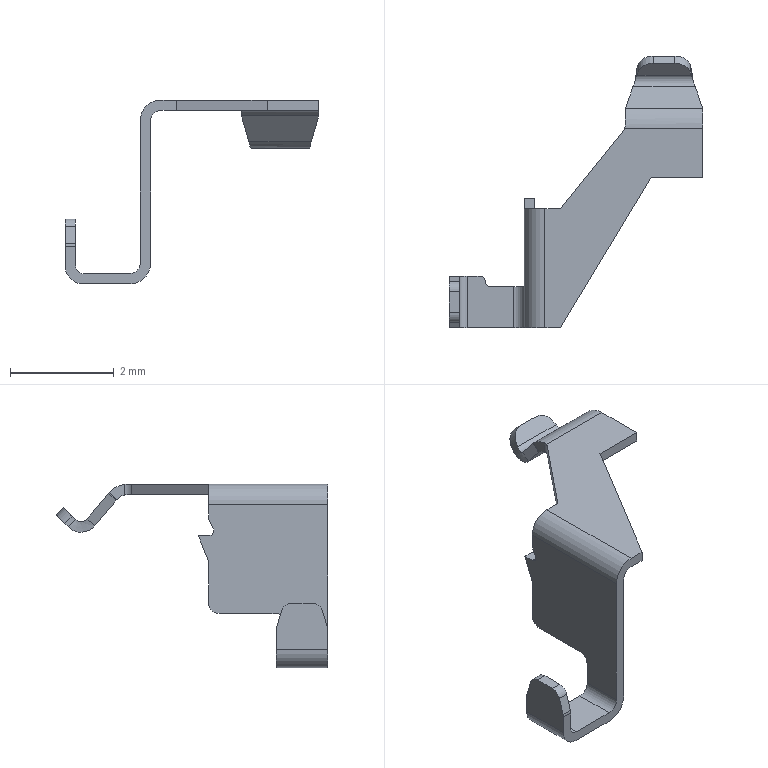Part | Creo | 1 solid | 60 faces | box 4.9 x 5.245 x 3.55 mm | volume 3.175 mm3 | plane 34 | cylinder 22 | spline 4 | commonest cylinder face diameters 0.4 x9 0.2 x3 0.6 x3 0.3 x2 0.7 x2 0.8 x2